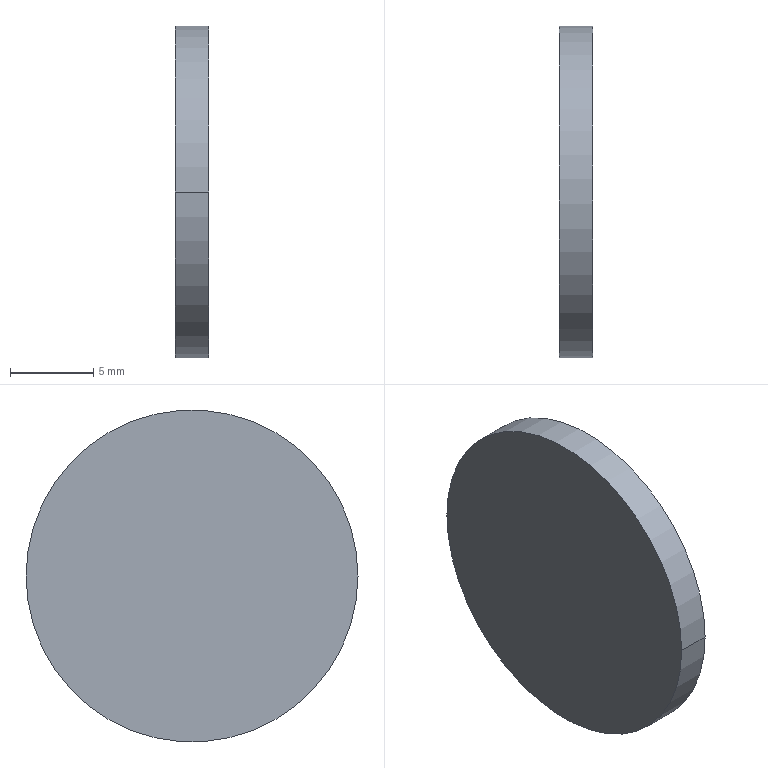Part | STEP file | _X2_7FC5724752A070ED7BA1_X0_1_6 | 1 solid | 4 faces | box 2 x 20 x 20 mm | volume 628.319 mm3 | cylinder 2 | plane 2 | commonest cylinder face diameters 20 x2
STEP:
#1=CARTESIAN_POINT('',(0.,0.,0.));
#2=DIRECTION('',(0.,0.,1.));
#3=DIRECTION('',(1.,0.,0.));
#4=AXIS2_PLACEMENT_3D('',#1,#2,#3);
#5=CARTESIAN_POINT('',(-22.,-10.,0.));
#6=VERTEX_POINT('',#5);
#7=CARTESIAN_POINT('',(-20.,-10.,0.));
#8=VERTEX_POINT('',#7);
#9=CARTESIAN_POINT('',(-22.,-10.,0.));
#10=DIRECTION('',(1.,0.,0.));
#11=VECTOR('',#10,1.);
#12=LINE('',#9,#11);
#13=CARTESIAN_POINT('',(-22.,0.,0.));
#14=DIRECTION('',(1.,0.,0.));
#15=DIRECTION('',(0.,1.,0.));
#16=AXIS2_PLACEMENT_3D('',#13,#14,#15);
#17=CYLINDRICAL_SURFACE('',#16,10.);
#18=CARTESIAN_POINT('',(3.142,0.));
#19=DIRECTION('',(0.,1.));
#20=VECTOR('',#19,1.);
#21=LINE('',#18,#20);
#22=(GEOMETRIC_REPRESENTATION_CONTEXT(2)PARAMETRIC_REPRESENTATION_CONTEXT()REPRESENTATION_CONTEXT('',''));
#23=DEFINITIONAL_REPRESENTATION('',(#21),#22);
#24=PCURVE('',#17,#23);
#25=CARTESIAN_POINT('',(-22.,0.,0.));
#26=DIRECTION('',(1.,0.,0.));
#27=DIRECTION('',(0.,1.,0.));
#28=AXIS2_PLACEMENT_3D('',#25,#26,#27);
#29=CYLINDRICAL_SURFACE('',#28,10.);
#30=CARTESIAN_POINT('',(3.142,0.));
#31=DIRECTION('',(0.,1.));
#32=VECTOR('',#31,1.);
#33=LINE('',#30,#32);
#34=(GEOMETRIC_REPRESENTATION_CONTEXT(2)PARAMETRIC_REPRESENTATION_CONTEXT()REPRESENTATION_CONTEXT('',''));
#35=DEFINITIONAL_REPRESENTATION('',(#33),#34);
#36=PCURVE('',#29,#35);
#37=SURFACE_CURVE('',#12,(#24,#36),.PCURVE_S1.);
#38=EDGE_CURVE('',#6,#8,#37,.T.);
#39=ORIENTED_EDGE('',*,*,#38,.T.);
#40=CARTESIAN_POINT('',(-20.,10.,0.));
#41=VERTEX_POINT('',#40);
#42=CARTESIAN_POINT('',(-20.,0.,0.));
#43=DIRECTION('',(1.,0.,0.));
#44=DIRECTION('',(0.,1.,0.));
#45=AXIS2_PLACEMENT_3D('',#42,#43,#44);
#46=CIRCLE('',#45,10.);
#47=CARTESIAN_POINT('',(0.,2.));
#48=DIRECTION('',(1.,0.));
#49=VECTOR('',#48,1.);
#50=LINE('',#47,#49);
#51=(GEOMETRIC_REPRESENTATION_CONTEXT(2)PARAMETRIC_REPRESENTATION_CONTEXT()REPRESENTATION_CONTEXT('',''));
#52=DEFINITIONAL_REPRESENTATION('',(#50),#51);
#53=PCURVE('',#17,#52);
#54=CARTESIAN_POINT('',(-20.,0.,0.));
#55=DIRECTION('',(-1.,0.,0.));
#56=DIRECTION('',(0.,-1.,0.));
#57=AXIS2_PLACEMENT_3D('',#54,#55,#56);
#58=PLANE('',#57);
#59=CARTESIAN_POINT('',(-10.,0.));
#60=CARTESIAN_POINT('',(-10.,17.321));
#61=CARTESIAN_POINT('',(5.,8.66));
#62=CARTESIAN_POINT('',(20.,0.));
#63=CARTESIAN_POINT('',(5.,-8.66));
#64=CARTESIAN_POINT('',(-10.,-17.321));
#65=CARTESIAN_POINT('',(-10.,0.));
#66=(BOUNDED_CURVE()B_SPLINE_CURVE(2,(#59,#60,#61,#62,#63,#64,#65),.UNSPECIFIED.,.T.,.F.)B_SPLINE_CURVE_WITH_KNOTS((1,2,2,2,2,1),(-2.094,0.,2.094,4.189,6.283,8.378),.UNSPECIFIED.)CURVE()GEOMETRIC_REPRESENTATION_ITEM()RATIONAL_B_SPLINE_CURVE((1.,0.5,1.,0.5,1.,0.5,1.))REPRESENTATION_ITEM(''));
#67=(GEOMETRIC_REPRESENTATION_CONTEXT(2)PARAMETRIC_REPRESENTATION_CONTEXT()REPRESENTATION_CONTEXT('',''));
#68=DEFINITIONAL_REPRESENTATION('',(#66),#67);
#69=PCURVE('',#58,#68);
#70=SURFACE_CURVE('',#46,(#53,#69),.PCURVE_S1.);
#71=EDGE_CURVE('',#41,#8,#70,.T.);
#72=ORIENTED_EDGE('',*,*,#71,.F.);
#73=CARTESIAN_POINT('',(-22.,10.,0.));
#74=VERTEX_POINT('',#73);
#75=CARTESIAN_POINT('',(-22.,10.,0.));
#76=DIRECTION('',(1.,0.,0.));
#77=VECTOR('',#76,1.);
#78=LINE('',#75,#77);
#79=CARTESIAN_POINT('',(0.,0.));
#80=DIRECTION('',(0.,1.));
#81=VECTOR('',#80,1.);
#82=LINE('',#79,#81);
#83=(GEOMETRIC_REPRESENTATION_CONTEXT(2)PARAMETRIC_REPRESENTATION_CONTEXT()REPRESENTATION_CONTEXT('',''));
#84=DEFINITIONAL_REPRESENTATION('',(#82),#83);
#85=PCURVE('',#17,#84);
#86=CARTESIAN_POINT('',(6.283,0.));
#87=DIRECTION('',(0.,1.));
#88=VECTOR('',#87,1.);
#89=LINE('',#86,#88);
#90=(GEOMETRIC_REPRESENTATION_CONTEXT(2)PARAMETRIC_REPRESENTATION_CONTEXT()REPRESENTATION_CONTEXT('',''));
#91=DEFINITIONAL_REPRESENTATION('',(#89),#90);
#92=PCURVE('',#29,#91);
#93=SURFACE_CURVE('',#78,(#85,#92),.PCURVE_S1.);
#94=EDGE_CURVE('',#74,#41,#93,.T.);
#95=ORIENTED_EDGE('',*,*,#94,.F.);
#96=CARTESIAN_POINT('',(-22.,0.,0.));
#97=DIRECTION('',(-1.,0.,0.));
#98=DIRECTION('',(0.,-1.,0.));
#99=AXIS2_PLACEMENT_3D('',#96,#97,#98);
#100=CIRCLE('',#99,10.);
#101=CARTESIAN_POINT('',(3.142,0.));
#102=DIRECTION('',(-1.,0.));
#103=VECTOR('',#102,1.);
#104=LINE('',#101,#103);
#105=(GEOMETRIC_REPRESENTATION_CONTEXT(2)PARAMETRIC_REPRESENTATION_CONTEXT()REPRESENTATION_CONTEXT('',''));
#106=DEFINITIONAL_REPRESENTATION('',(#104),#105);
#107=PCURVE('',#17,#106);
#108=CARTESIAN_POINT('',(-22.,0.,0.));
#109=DIRECTION('',(-1.,0.,0.));
#110=DIRECTION('',(0.,-1.,0.));
#111=AXIS2_PLACEMENT_3D('',#108,#109,#110);
#112=PLANE('',#111);
#113=CARTESIAN_POINT('',(0.,0.));
#114=DIRECTION('',(1.,0.));
#115=AXIS2_PLACEMENT_2D('',#113,#114);
#116=CIRCLE('',#115,10.);
#117=(GEOMETRIC_REPRESENTATION_CONTEXT(2)PARAMETRIC_REPRESENTATION_CONTEXT()REPRESENTATION_CONTEXT('',''));
#118=DEFINITIONAL_REPRESENTATION('',(#116),#117);
#119=PCURVE('',#112,#118);
#120=SURFACE_CURVE('',#100,(#107,#119),.PCURVE_S1.);
#121=EDGE_CURVE('',#6,#74,#120,.T.);
#122=ORIENTED_EDGE('',*,*,#121,.F.);
#123=EDGE_LOOP('',(#39,#72,#95,#122));
#124=FACE_BOUND('',#123,.T.);
#125=ADVANCED_FACE('',(#124),#17,.T.);
#126=ORIENTED_EDGE('',*,*,#121,.F.);
#127=CARTESIAN_POINT('',(-22.,0.,0.));
#128=DIRECTION('',(-1.,0.,0.));
#129=DIRECTION('',(0.,1.,0.));
#130=AXIS2_PLACEMENT_3D('',#127,#128,#129);
#131=CIRCLE('',#130,10.);
#132=CARTESIAN_POINT('',(0.,0.));
#133=DIRECTION('',(-1.,0.));
#134=AXIS2_PLACEMENT_2D('',#132,#133);
#135=CIRCLE('',#134,10.);
#136=(GEOMETRIC_REPRESENTATION_CONTEXT(2)PARAMETRIC_REPRESENTATION_CONTEXT()REPRESENTATION_CONTEXT('',''));
#137=DEFINITIONAL_REPRESENTATION('',(#135),#136);
#138=PCURVE('',#112,#137);
#139=CARTESIAN_POINT('',(6.283,0.));
#140=DIRECTION('',(-1.,0.));
#141=VECTOR('',#140,1.);
#142=LINE('',#139,#141);
#143=(GEOMETRIC_REPRESENTATION_CONTEXT(2)PARAMETRIC_REPRESENTATION_CONTEXT()REPRESENTATION_CONTEXT('',''));
#144=DEFINITIONAL_REPRESENTATION('',(#142),#143);
#145=PCURVE('',#29,#144);
#146=SURFACE_CURVE('',#131,(#138,#145),.PCURVE_S1.);
#147=EDGE_CURVE('',#74,#6,#146,.T.);
#148=ORIENTED_EDGE('',*,*,#147,.F.);
#149=EDGE_LOOP('',(#126,#148));
#150=FACE_BOUND('',#149,.F.);
#151=ADVANCED_FACE('',(#150),#112,.T.);
#152=ORIENTED_EDGE('',*,*,#94,.T.);
#153=CARTESIAN_POINT('',(-20.,0.,0.));
#154=DIRECTION('',(1.,0.,0.));
#155=DIRECTION('',(0.,-1.,0.));
#156=AXIS2_PLACEMENT_3D('',#153,#154,#155);
#157=CIRCLE('',#156,10.);
#158=CARTESIAN_POINT('',(3.142,2.));
#159=DIRECTION('',(1.,0.));
#160=VECTOR('',#159,1.);
#161=LINE('',#158,#160);
#162=(GEOMETRIC_REPRESENTATION_CONTEXT(2)PARAMETRIC_REPRESENTATION_CONTEXT()REPRESENTATION_CONTEXT('',''));
#163=DEFINITIONAL_REPRESENTATION('',(#161),#162);
#164=PCURVE('',#29,#163);
#165=CARTESIAN_POINT('',(10.,0.));
#166=CARTESIAN_POINT('',(10.,-17.321));
#167=CARTESIAN_POINT('',(-5.,-8.66));
#168=CARTESIAN_POINT('',(-20.,0.));
#169=CARTESIAN_POINT('',(-5.,8.66));
#170=CARTESIAN_POINT('',(10.,17.321));
#171=CARTESIAN_POINT('',(10.,0.));
#172=(BOUNDED_CURVE()B_SPLINE_CURVE(2,(#165,#166,#167,#168,#169,#170,#171),.UNSPECIFIED.,.T.,.F.)B_SPLINE_CURVE_WITH_KNOTS((1,2,2,2,2,1),(-2.094,0.,2.094,4.189,6.283,8.378),.UNSPECIFIED.)CURVE()GEOMETRIC_REPRESENTATION_ITEM()RATIONAL_B_SPLINE_CURVE((1.,0.5,1.,0.5,1.,0.5,1.))REPRESENTATION_ITEM(''));
#173=(GEOMETRIC_REPRESENTATION_CONTEXT(2)PARAMETRIC_REPRESENTATION_CONTEXT()REPRESENTATION_CONTEXT('',''));
#174=DEFINITIONAL_REPRESENTATION('',(#172),#173);
#175=PCURVE('',#58,#174);
#176=SURFACE_CURVE('',#157,(#164,#175),.PCURVE_S1.);
#177=EDGE_CURVE('',#8,#41,#176,.T.);
#178=ORIENTED_EDGE('',*,*,#177,.F.);
#179=ORIENTED_EDGE('',*,*,#38,.F.);
#180=ORIENTED_EDGE('',*,*,#147,.F.);
#181=EDGE_LOOP('',(#152,#178,#179,#180));
#182=FACE_BOUND('',#181,.T.);
#183=ADVANCED_FACE('',(#182),#29,.T.);
#184=ORIENTED_EDGE('',*,*,#177,.F.);
#185=ORIENTED_EDGE('',*,*,#71,.F.);
#186=EDGE_LOOP('',(#184,#185));
#187=FACE_BOUND('',#186,.F.);
#188=ADVANCED_FACE('',(#187),#58,.F.);
#189=CLOSED_SHELL('',(#125,#151,#183,#188));
#190=MANIFOLD_SOLID_BREP('',#189);
#191=(LENGTH_UNIT()NAMED_UNIT(*)SI_UNIT(.MILLI.,.METRE.));
#192=UNCERTAINTY_MEASURE_WITH_UNIT(LENGTH_MEASURE(0.0000001),#191,'','');
#193=(NAMED_UNIT(*)PLANE_ANGLE_UNIT()SI_UNIT($,.RADIAN.));
#194=(NAMED_UNIT(*)SI_UNIT($,.STERADIAN.)SOLID_ANGLE_UNIT());
#195=(GEOMETRIC_REPRESENTATION_CONTEXT(3)GLOBAL_UNCERTAINTY_ASSIGNED_CONTEXT((#192))GLOBAL_UNIT_ASSIGNED_CONTEXT((#191,#193,#194))REPRESENTATION_CONTEXT('',''));
#196=ADVANCED_BREP_SHAPE_REPRESENTATION('',(#4,#190),#195);